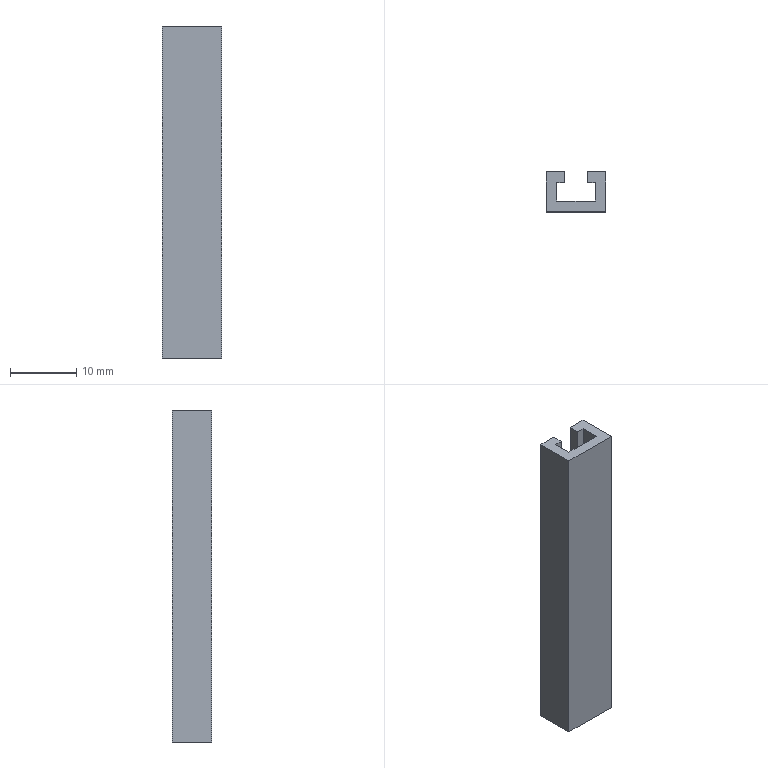Part | SolidWorks | features Extrusion 1 | 1 solid | 14 faces | box 9 x 6 x 50 mm | volume 1608 mm3 | plane 14
STEP:
#1=CARTESIAN_POINT('',(4.5,0.,-25.));
#2=VERTEX_POINT('',#1);
#3=CARTESIAN_POINT('',(4.5,6.,-25.));
#4=VERTEX_POINT('',#3);
#5=CARTESIAN_POINT('',(4.5,6.,-25.));
#6=DIRECTION('',(0.,1.,0.));
#7=VECTOR('',#6,1000.);
#8=LINE('',#5,#7);
#9=EDGE_CURVE('',#2,#4,#8,.T.);
#10=ORIENTED_EDGE('',*,*,#9,.T.);
#11=CARTESIAN_POINT('',(4.5,6.,25.));
#12=VERTEX_POINT('',#11);
#13=CARTESIAN_POINT('',(4.5,6.,25.));
#14=DIRECTION('',(0.,0.,-1.));
#15=VECTOR('',#14,1000.);
#16=LINE('',#13,#15);
#17=EDGE_CURVE('',#12,#4,#16,.T.);
#18=ORIENTED_EDGE('',*,*,#17,.F.);
#19=CARTESIAN_POINT('',(4.5,0.,25.));
#20=VERTEX_POINT('',#19);
#21=CARTESIAN_POINT('',(4.5,6.,25.));
#22=DIRECTION('',(0.,1.,0.));
#23=VECTOR('',#22,1000.);
#24=LINE('',#21,#23);
#25=EDGE_CURVE('',#20,#12,#24,.T.);
#26=ORIENTED_EDGE('',*,*,#25,.F.);
#27=CARTESIAN_POINT('',(4.5,0.,25.));
#28=DIRECTION('',(0.,0.,-1.));
#29=VECTOR('',#28,1000.);
#30=LINE('',#27,#29);
#31=EDGE_CURVE('',#20,#2,#30,.T.);
#32=ORIENTED_EDGE('',*,*,#31,.T.);
#33=EDGE_LOOP('',(#10,#18,#26,#32));
#34=FACE_OUTER_BOUND('',#33,.T.);
#35=CARTESIAN_POINT('',(4.5,6.,25.));
#36=DIRECTION('',(-1.,0.,0.));
#37=DIRECTION('',(0.,0.,1.));
#38=AXIS2_PLACEMENT_3D('',#35,#36,#37);
#39=PLANE('',#38);
#40=ADVANCED_FACE('',(#34),#39,.F.);
#41=CARTESIAN_POINT('',(1.75,6.,-25.));
#42=VERTEX_POINT('',#41);
#43=CARTESIAN_POINT('',(1.75,6.,-25.));
#44=DIRECTION('',(-1.,0.,0.));
#45=VECTOR('',#44,1000.);
#46=LINE('',#43,#45);
#47=EDGE_CURVE('',#4,#42,#46,.T.);
#48=ORIENTED_EDGE('',*,*,#47,.T.);
#49=CARTESIAN_POINT('',(1.75,6.,25.));
#50=VERTEX_POINT('',#49);
#51=CARTESIAN_POINT('',(1.75,6.,25.));
#52=DIRECTION('',(0.,0.,-1.));
#53=VECTOR('',#52,1000.);
#54=LINE('',#51,#53);
#55=EDGE_CURVE('',#50,#42,#54,.T.);
#56=ORIENTED_EDGE('',*,*,#55,.F.);
#57=CARTESIAN_POINT('',(1.75,6.,25.));
#58=DIRECTION('',(-1.,0.,0.));
#59=VECTOR('',#58,1000.);
#60=LINE('',#57,#59);
#61=EDGE_CURVE('',#12,#50,#60,.T.);
#62=ORIENTED_EDGE('',*,*,#61,.F.);
#63=ORIENTED_EDGE('',*,*,#17,.T.);
#64=EDGE_LOOP('',(#48,#56,#62,#63));
#65=FACE_OUTER_BOUND('',#64,.T.);
#66=CARTESIAN_POINT('',(1.75,6.,25.));
#67=DIRECTION('',(0.,-1.,0.));
#68=DIRECTION('',(0.,0.,-1.));
#69=AXIS2_PLACEMENT_3D('',#66,#67,#68);
#70=PLANE('',#69);
#71=ADVANCED_FACE('',(#65),#70,.F.);
#72=CARTESIAN_POINT('',(1.75,4.4,-25.));
#73=VERTEX_POINT('',#72);
#74=CARTESIAN_POINT('',(1.75,4.4,-25.));
#75=DIRECTION('',(0.,-1.,0.));
#76=VECTOR('',#75,1000.);
#77=LINE('',#74,#76);
#78=EDGE_CURVE('',#42,#73,#77,.T.);
#79=ORIENTED_EDGE('',*,*,#78,.T.);
#80=CARTESIAN_POINT('',(1.75,4.4,25.));
#81=VERTEX_POINT('',#80);
#82=CARTESIAN_POINT('',(1.75,4.4,25.));
#83=DIRECTION('',(0.,0.,-1.));
#84=VECTOR('',#83,1000.);
#85=LINE('',#82,#84);
#86=EDGE_CURVE('',#81,#73,#85,.T.);
#87=ORIENTED_EDGE('',*,*,#86,.F.);
#88=CARTESIAN_POINT('',(1.75,4.4,25.));
#89=DIRECTION('',(0.,-1.,0.));
#90=VECTOR('',#89,1000.);
#91=LINE('',#88,#90);
#92=EDGE_CURVE('',#50,#81,#91,.T.);
#93=ORIENTED_EDGE('',*,*,#92,.F.);
#94=ORIENTED_EDGE('',*,*,#55,.T.);
#95=EDGE_LOOP('',(#79,#87,#93,#94));
#96=FACE_OUTER_BOUND('',#95,.T.);
#97=CARTESIAN_POINT('',(1.75,4.4,25.));
#98=DIRECTION('',(1.,0.,0.));
#99=DIRECTION('',(0.,0.,-1.));
#100=AXIS2_PLACEMENT_3D('',#97,#98,#99);
#101=PLANE('',#100);
#102=ADVANCED_FACE('',(#96),#101,.F.);
#103=CARTESIAN_POINT('',(2.9,4.4,-25.));
#104=VERTEX_POINT('',#103);
#105=CARTESIAN_POINT('',(2.9,4.4,-25.));
#106=DIRECTION('',(1.,0.,0.));
#107=VECTOR('',#106,1000.);
#108=LINE('',#105,#107);
#109=EDGE_CURVE('',#73,#104,#108,.T.);
#110=ORIENTED_EDGE('',*,*,#109,.T.);
#111=CARTESIAN_POINT('',(2.9,4.4,25.));
#112=VERTEX_POINT('',#111);
#113=CARTESIAN_POINT('',(2.9,4.4,25.));
#114=DIRECTION('',(0.,0.,-1.));
#115=VECTOR('',#114,1000.);
#116=LINE('',#113,#115);
#117=EDGE_CURVE('',#112,#104,#116,.T.);
#118=ORIENTED_EDGE('',*,*,#117,.F.);
#119=CARTESIAN_POINT('',(2.9,4.4,25.));
#120=DIRECTION('',(1.,0.,0.));
#121=VECTOR('',#120,1000.);
#122=LINE('',#119,#121);
#123=EDGE_CURVE('',#81,#112,#122,.T.);
#124=ORIENTED_EDGE('',*,*,#123,.F.);
#125=ORIENTED_EDGE('',*,*,#86,.T.);
#126=EDGE_LOOP('',(#110,#118,#124,#125));
#127=FACE_OUTER_BOUND('',#126,.T.);
#128=CARTESIAN_POINT('',(2.9,4.4,25.));
#129=DIRECTION('',(0.,1.,0.));
#130=DIRECTION('',(0.,0.,1.));
#131=AXIS2_PLACEMENT_3D('',#128,#129,#130);
#132=PLANE('',#131);
#133=ADVANCED_FACE('',(#127),#132,.F.);
#134=CARTESIAN_POINT('',(2.9,1.6,-25.));
#135=VERTEX_POINT('',#134);
#136=CARTESIAN_POINT('',(2.9,1.6,-25.));
#137=DIRECTION('',(0.,-1.,0.));
#138=VECTOR('',#137,1000.);
#139=LINE('',#136,#138);
#140=EDGE_CURVE('',#104,#135,#139,.T.);
#141=ORIENTED_EDGE('',*,*,#140,.T.);
#142=CARTESIAN_POINT('',(2.9,1.6,25.));
#143=VERTEX_POINT('',#142);
#144=CARTESIAN_POINT('',(2.9,1.6,25.));
#145=DIRECTION('',(0.,0.,-1.));
#146=VECTOR('',#145,1000.);
#147=LINE('',#144,#146);
#148=EDGE_CURVE('',#143,#135,#147,.T.);
#149=ORIENTED_EDGE('',*,*,#148,.F.);
#150=CARTESIAN_POINT('',(2.9,1.6,25.));
#151=DIRECTION('',(0.,-1.,0.));
#152=VECTOR('',#151,1000.);
#153=LINE('',#150,#152);
#154=EDGE_CURVE('',#112,#143,#153,.T.);
#155=ORIENTED_EDGE('',*,*,#154,.F.);
#156=ORIENTED_EDGE('',*,*,#117,.T.);
#157=EDGE_LOOP('',(#141,#149,#155,#156));
#158=FACE_OUTER_BOUND('',#157,.T.);
#159=CARTESIAN_POINT('',(2.9,1.6,25.));
#160=DIRECTION('',(1.,0.,0.));
#161=DIRECTION('',(0.,0.,-1.));
#162=AXIS2_PLACEMENT_3D('',#159,#160,#161);
#163=PLANE('',#162);
#164=ADVANCED_FACE('',(#158),#163,.F.);
#165=CARTESIAN_POINT('',(-2.9,1.6,-25.));
#166=VERTEX_POINT('',#165);
#167=CARTESIAN_POINT('',(-2.9,1.6,-25.));
#168=DIRECTION('',(-1.,0.,0.));
#169=VECTOR('',#168,1000.);
#170=LINE('',#167,#169);
#171=EDGE_CURVE('',#135,#166,#170,.T.);
#172=ORIENTED_EDGE('',*,*,#171,.T.);
#173=CARTESIAN_POINT('',(-2.9,1.6,25.));
#174=VERTEX_POINT('',#173);
#175=CARTESIAN_POINT('',(-2.9,1.6,25.));
#176=DIRECTION('',(0.,0.,-1.));
#177=VECTOR('',#176,1000.);
#178=LINE('',#175,#177);
#179=EDGE_CURVE('',#174,#166,#178,.T.);
#180=ORIENTED_EDGE('',*,*,#179,.F.);
#181=CARTESIAN_POINT('',(-2.9,1.6,25.));
#182=DIRECTION('',(-1.,0.,0.));
#183=VECTOR('',#182,1000.);
#184=LINE('',#181,#183);
#185=EDGE_CURVE('',#143,#174,#184,.T.);
#186=ORIENTED_EDGE('',*,*,#185,.F.);
#187=ORIENTED_EDGE('',*,*,#148,.T.);
#188=EDGE_LOOP('',(#172,#180,#186,#187));
#189=FACE_OUTER_BOUND('',#188,.T.);
#190=CARTESIAN_POINT('',(-2.9,1.6,25.));
#191=DIRECTION('',(0.,-1.,0.));
#192=DIRECTION('',(0.,0.,-1.));
#193=AXIS2_PLACEMENT_3D('',#190,#191,#192);
#194=PLANE('',#193);
#195=ADVANCED_FACE('',(#189),#194,.F.);
#196=CARTESIAN_POINT('',(-2.9,4.4,-25.));
#197=VERTEX_POINT('',#196);
#198=CARTESIAN_POINT('',(-2.9,4.4,-25.));
#199=DIRECTION('',(0.,1.,0.));
#200=VECTOR('',#199,1000.);
#201=LINE('',#198,#200);
#202=EDGE_CURVE('',#166,#197,#201,.T.);
#203=ORIENTED_EDGE('',*,*,#202,.T.);
#204=CARTESIAN_POINT('',(-2.9,4.4,25.));
#205=VERTEX_POINT('',#204);
#206=CARTESIAN_POINT('',(-2.9,4.4,25.));
#207=DIRECTION('',(0.,0.,-1.));
#208=VECTOR('',#207,1000.);
#209=LINE('',#206,#208);
#210=EDGE_CURVE('',#205,#197,#209,.T.);
#211=ORIENTED_EDGE('',*,*,#210,.F.);
#212=CARTESIAN_POINT('',(-2.9,4.4,25.));
#213=DIRECTION('',(0.,1.,0.));
#214=VECTOR('',#213,1000.);
#215=LINE('',#212,#214);
#216=EDGE_CURVE('',#174,#205,#215,.T.);
#217=ORIENTED_EDGE('',*,*,#216,.F.);
#218=ORIENTED_EDGE('',*,*,#179,.T.);
#219=EDGE_LOOP('',(#203,#211,#217,#218));
#220=FACE_OUTER_BOUND('',#219,.T.);
#221=CARTESIAN_POINT('',(-2.9,4.4,25.));
#222=DIRECTION('',(-1.,0.,0.));
#223=DIRECTION('',(0.,-1.,0.));
#224=AXIS2_PLACEMENT_3D('',#221,#222,#223);
#225=PLANE('',#224);
#226=ADVANCED_FACE('',(#220),#225,.F.);
#227=CARTESIAN_POINT('',(-1.75,4.4,-25.));
#228=VERTEX_POINT('',#227);
#229=CARTESIAN_POINT('',(-1.75,4.4,-25.));
#230=DIRECTION('',(1.,0.,0.));
#231=VECTOR('',#230,1000.);
#232=LINE('',#229,#231);
#233=EDGE_CURVE('',#197,#228,#232,.T.);
#234=ORIENTED_EDGE('',*,*,#233,.T.);
#235=CARTESIAN_POINT('',(-1.75,4.4,25.));
#236=VERTEX_POINT('',#235);
#237=CARTESIAN_POINT('',(-1.75,4.4,25.));
#238=DIRECTION('',(0.,0.,-1.));
#239=VECTOR('',#238,1000.);
#240=LINE('',#237,#239);
#241=EDGE_CURVE('',#236,#228,#240,.T.);
#242=ORIENTED_EDGE('',*,*,#241,.F.);
#243=CARTESIAN_POINT('',(-1.75,4.4,25.));
#244=DIRECTION('',(1.,0.,0.));
#245=VECTOR('',#244,1000.);
#246=LINE('',#243,#245);
#247=EDGE_CURVE('',#205,#236,#246,.T.);
#248=ORIENTED_EDGE('',*,*,#247,.F.);
#249=ORIENTED_EDGE('',*,*,#210,.T.);
#250=EDGE_LOOP('',(#234,#242,#248,#249));
#251=FACE_OUTER_BOUND('',#250,.T.);
#252=CARTESIAN_POINT('',(-1.75,4.4,25.));
#253=DIRECTION('',(0.,1.,0.));
#254=DIRECTION('',(0.,0.,1.));
#255=AXIS2_PLACEMENT_3D('',#252,#253,#254);
#256=PLANE('',#255);
#257=ADVANCED_FACE('',(#251),#256,.F.);
#258=CARTESIAN_POINT('',(-1.75,6.,-25.));
#259=VERTEX_POINT('',#258);
#260=CARTESIAN_POINT('',(-1.75,6.,-25.));
#261=DIRECTION('',(0.,1.,0.));
#262=VECTOR('',#261,1000.);
#263=LINE('',#260,#262);
#264=EDGE_CURVE('',#228,#259,#263,.T.);
#265=ORIENTED_EDGE('',*,*,#264,.T.);
#266=CARTESIAN_POINT('',(-1.75,6.,25.));
#267=VERTEX_POINT('',#266);
#268=CARTESIAN_POINT('',(-1.75,6.,25.));
#269=DIRECTION('',(0.,0.,-1.));
#270=VECTOR('',#269,1000.);
#271=LINE('',#268,#270);
#272=EDGE_CURVE('',#267,#259,#271,.T.);
#273=ORIENTED_EDGE('',*,*,#272,.F.);
#274=CARTESIAN_POINT('',(-1.75,6.,25.));
#275=DIRECTION('',(0.,1.,0.));
#276=VECTOR('',#275,1000.);
#277=LINE('',#274,#276);
#278=EDGE_CURVE('',#236,#267,#277,.T.);
#279=ORIENTED_EDGE('',*,*,#278,.F.);
#280=ORIENTED_EDGE('',*,*,#241,.T.);
#281=EDGE_LOOP('',(#265,#273,#279,#280));
#282=FACE_OUTER_BOUND('',#281,.T.);
#283=CARTESIAN_POINT('',(-1.75,6.,25.));
#284=DIRECTION('',(-1.,0.,0.));
#285=DIRECTION('',(0.,0.,1.));
#286=AXIS2_PLACEMENT_3D('',#283,#284,#285);
#287=PLANE('',#286);
#288=ADVANCED_FACE('',(#282),#287,.F.);
#289=CARTESIAN_POINT('',(-4.5,6.,-25.));
#290=VERTEX_POINT('',#289);
#291=CARTESIAN_POINT('',(-4.5,6.,-25.));
#292=DIRECTION('',(-1.,0.,0.));
#293=VECTOR('',#292,1000.);
#294=LINE('',#291,#293);
#295=EDGE_CURVE('',#259,#290,#294,.T.);
#296=ORIENTED_EDGE('',*,*,#295,.T.);
#297=CARTESIAN_POINT('',(-4.5,6.,25.));
#298=VERTEX_POINT('',#297);
#299=CARTESIAN_POINT('',(-4.5,6.,25.));
#300=DIRECTION('',(0.,0.,-1.));
#301=VECTOR('',#300,1000.);
#302=LINE('',#299,#301);
#303=EDGE_CURVE('',#298,#290,#302,.T.);
#304=ORIENTED_EDGE('',*,*,#303,.F.);
#305=CARTESIAN_POINT('',(-4.5,6.,25.));
#306=DIRECTION('',(-1.,0.,0.));
#307=VECTOR('',#306,1000.);
#308=LINE('',#305,#307);
#309=EDGE_CURVE('',#267,#298,#308,.T.);
#310=ORIENTED_EDGE('',*,*,#309,.F.);
#311=ORIENTED_EDGE('',*,*,#272,.T.);
#312=EDGE_LOOP('',(#296,#304,#310,#311));
#313=FACE_OUTER_BOUND('',#312,.T.);
#314=CARTESIAN_POINT('',(-4.5,6.,25.));
#315=DIRECTION('',(0.,-1.,0.));
#316=DIRECTION('',(0.,0.,-1.));
#317=AXIS2_PLACEMENT_3D('',#314,#315,#316);
#318=PLANE('',#317);
#319=ADVANCED_FACE('',(#313),#318,.F.);
#320=CARTESIAN_POINT('',(-4.5,0.,-25.));
#321=VERTEX_POINT('',#320);
#322=CARTESIAN_POINT('',(-4.5,0.,-25.));
#323=DIRECTION('',(0.,-1.,0.));
#324=VECTOR('',#323,1000.);
#325=LINE('',#322,#324);
#326=EDGE_CURVE('',#290,#321,#325,.T.);
#327=ORIENTED_EDGE('',*,*,#326,.T.);
#328=CARTESIAN_POINT('',(-4.5,0.,25.));
#329=VERTEX_POINT('',#328);
#330=CARTESIAN_POINT('',(-4.5,0.,25.));
#331=DIRECTION('',(0.,0.,-1.));
#332=VECTOR('',#331,1000.);
#333=LINE('',#330,#332);
#334=EDGE_CURVE('',#329,#321,#333,.T.);
#335=ORIENTED_EDGE('',*,*,#334,.F.);
#336=CARTESIAN_POINT('',(-4.5,0.,25.));
#337=DIRECTION('',(0.,-1.,0.));
#338=VECTOR('',#337,1000.);
#339=LINE('',#336,#338);
#340=EDGE_CURVE('',#298,#329,#339,.T.);
#341=ORIENTED_EDGE('',*,*,#340,.F.);
#342=ORIENTED_EDGE('',*,*,#303,.T.);
#343=EDGE_LOOP('',(#327,#335,#341,#342));
#344=FACE_OUTER_BOUND('',#343,.T.);
#345=CARTESIAN_POINT('',(-4.5,0.,25.));
#346=DIRECTION('',(1.,0.,0.));
#347=DIRECTION('',(0.,0.,-1.));
#348=AXIS2_PLACEMENT_3D('',#345,#346,#347);
#349=PLANE('',#348);
#350=ADVANCED_FACE('',(#344),#349,.F.);
#351=CARTESIAN_POINT('',(0.,0.,-25.));
#352=DIRECTION('',(1.,0.,0.));
#353=VECTOR('',#352,1000.);
#354=LINE('',#351,#353);
#355=EDGE_CURVE('',#321,#2,#354,.T.);
#356=ORIENTED_EDGE('',*,*,#355,.T.);
#357=ORIENTED_EDGE('',*,*,#31,.F.);
#358=CARTESIAN_POINT('',(4.5,0.,25.));
#359=DIRECTION('',(1.,0.,0.));
#360=VECTOR('',#359,1000.);
#361=LINE('',#358,#360);
#362=EDGE_CURVE('',#329,#20,#361,.T.);
#363=ORIENTED_EDGE('',*,*,#362,.F.);
#364=ORIENTED_EDGE('',*,*,#334,.T.);
#365=EDGE_LOOP('',(#356,#357,#363,#364));
#366=FACE_OUTER_BOUND('',#365,.T.);
#367=CARTESIAN_POINT('',(0.,0.,25.));
#368=DIRECTION('',(0.,1.,0.));
#369=DIRECTION('',(-1.,0.,0.));
#370=AXIS2_PLACEMENT_3D('',#367,#368,#369);
#371=PLANE('',#370);
#372=ADVANCED_FACE('',(#366),#371,.F.);
#373=ORIENTED_EDGE('',*,*,#362,.T.);
#374=ORIENTED_EDGE('',*,*,#25,.T.);
#375=ORIENTED_EDGE('',*,*,#61,.T.);
#376=ORIENTED_EDGE('',*,*,#92,.T.);
#377=ORIENTED_EDGE('',*,*,#123,.T.);
#378=ORIENTED_EDGE('',*,*,#154,.T.);
#379=ORIENTED_EDGE('',*,*,#185,.T.);
#380=ORIENTED_EDGE('',*,*,#216,.T.);
#381=ORIENTED_EDGE('',*,*,#247,.T.);
#382=ORIENTED_EDGE('',*,*,#278,.T.);
#383=ORIENTED_EDGE('',*,*,#309,.T.);
#384=ORIENTED_EDGE('',*,*,#340,.T.);
#385=EDGE_LOOP('',(#373,#374,#375,#376,#377,#378,#379,#380,#381,#382,#383,#384));
#386=FACE_OUTER_BOUND('',#385,.T.);
#387=CARTESIAN_POINT('',(0.,0.,25.));
#388=DIRECTION('',(0.,0.,-1.));
#389=DIRECTION('',(-1.,0.,0.));
#390=AXIS2_PLACEMENT_3D('',#387,#388,#389);
#391=PLANE('',#390);
#392=ADVANCED_FACE('',(#386),#391,.F.);
#393=ORIENTED_EDGE('',*,*,#9,.F.);
#394=ORIENTED_EDGE('',*,*,#355,.F.);
#395=ORIENTED_EDGE('',*,*,#326,.F.);
#396=ORIENTED_EDGE('',*,*,#295,.F.);
#397=ORIENTED_EDGE('',*,*,#264,.F.);
#398=ORIENTED_EDGE('',*,*,#233,.F.);
#399=ORIENTED_EDGE('',*,*,#202,.F.);
#400=ORIENTED_EDGE('',*,*,#171,.F.);
#401=ORIENTED_EDGE('',*,*,#140,.F.);
#402=ORIENTED_EDGE('',*,*,#109,.F.);
#403=ORIENTED_EDGE('',*,*,#78,.F.);
#404=ORIENTED_EDGE('',*,*,#47,.F.);
#405=EDGE_LOOP('',(#393,#394,#395,#396,#397,#398,#399,#400,#401,#402,#403,#404));
#406=FACE_OUTER_BOUND('',#405,.T.);
#407=CARTESIAN_POINT('',(0.,0.,-25.));
#408=DIRECTION('',(0.,0.,-1.));
#409=DIRECTION('',(-1.,0.,0.));
#410=AXIS2_PLACEMENT_3D('',#407,#408,#409);
#411=PLANE('',#410);
#412=ADVANCED_FACE('',(#406),#411,.T.);
#413=CLOSED_SHELL('',(#40,#71,#102,#133,#164,#195,#226,#257,#288,#319,#350,#372,#392,#412));
#414=MANIFOLD_SOLID_BREP('',#413);
#415=CARTESIAN_POINT('',(0.,0.,0.));
#416=DIRECTION('',(0.,0.,1.));
#417=DIRECTION('',(1.,0.,0.));
#418=AXIS2_PLACEMENT_3D('',#415,#416,#417);
#419=(LENGTH_UNIT()NAMED_UNIT(*)SI_UNIT(.MILLI.,.METRE.));
#420=UNCERTAINTY_MEASURE_WITH_UNIT(LENGTH_MEASURE(0.00001),#419,'','');
#421=(NAMED_UNIT(*)PLANE_ANGLE_UNIT()SI_UNIT($,.RADIAN.));
#422=(NAMED_UNIT(*)SI_UNIT($,.STERADIAN.)SOLID_ANGLE_UNIT());
#423=(GEOMETRIC_REPRESENTATION_CONTEXT(3)GLOBAL_UNCERTAINTY_ASSIGNED_CONTEXT((#420))GLOBAL_UNIT_ASSIGNED_CONTEXT((#419,#421,#422))REPRESENTATION_CONTEXT('',''));
#424=ADVANCED_BREP_SHAPE_REPRESENTATION('',(#414,#418),#423);